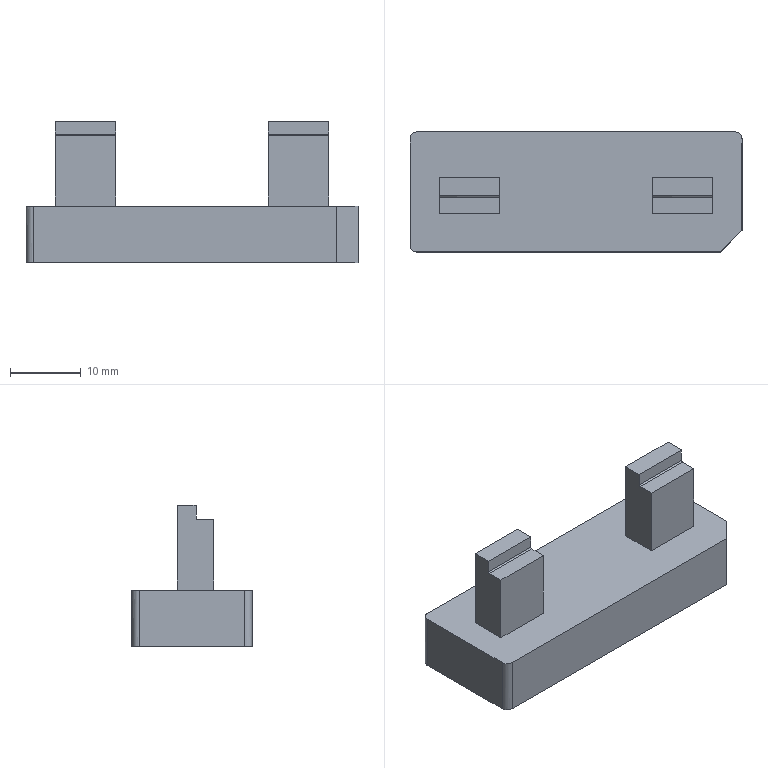NC program | PowerMill | posted by the shop | part box 47 x 17 x 19.985 mm
Lines 10964 to 11898 of 62704:
( TOOL ID   D10_1_1_1 )
( TOOL DIA. 10. TIP RAD 0 LENGTH 75.16 )
( Z = -2.265 )
T3 M6
T14
G91 G28 Z0
G0 G90 G54
M08
S8500 M3
X0 Y0 M8
G43 Z11.805 H3
X-.07 Y-.853
Z-1.065
G1 Z-2.265 F360
X-5.345 Y-.906 F600
G3 X-5.466 Y-1.223 I.478 J-.363
G1 X-5.474 Y-1.325
X-5.509 Y-1.6
X-5.56 Y-1.875
X-5.632 Y-2.177
X-5.706 Y-2.425
X-5.804 Y-2.7
X-5.918 Y-2.975
X-6.039 Y-3.227
X-6.177 Y-3.478
X-6.38 Y-3.8
X-6.581 Y-4.075
X-6.739 Y-4.268
X-6.814 Y-4.355
X-7.074 Y-4.625
X-7.3 Y-4.833
X-7.52 Y-5.013
X-7.739 Y-5.176
X-7.862 Y-5.259
X-8.143 Y-5.433
X-8.423 Y-5.583
X-8.734 Y-5.726
X-8.985 Y-5.824
X-9.266 Y-5.918
X-9.547 Y-5.995
X-9.827 Y-6.056
X-10.108 Y-6.101
X-10.389 Y-6.131
X-10.67 Y-6.146
X-19.374 Y-6.149
X-19.655 Y-6.139
X-19.935 Y-6.114
X-20.216 Y-6.074
X-20.497 Y-6.02
X-20.778 Y-5.949
X-21.059 Y-5.862
X-21.416 Y-5.726
X-21.658 Y-5.617
X-21.901 Y-5.492
X-22.156 Y-5.344
X-22.463 Y-5.139
X-22.743 Y-4.923
X-23.076 Y-4.625
X-23.339 Y-4.35
X-23.586 Y-4.054
X-23.777 Y-3.789
X-23.945 Y-3.525
X-24.099 Y-3.25
X-24.177 Y-3.093
X-24.249 Y-2.933
X-24.347 Y-2.697
X-24.444 Y-2.425
X-24.525 Y-2.15
X-24.563 Y-1.988
G3 X-24.805 Y-1.634 I-.584 J-.139
G0 Z4.005
G1 X-12.997 Y-11.339 F10000
G0 Z.935
G1 Z-.265 F360
X-12.996 Y-6.064 F600
X-12.957 Y-1.957
X-12.492 Y-1.961
G3 X-11.93 Y1.925 I.019 J1.981
G1 X-16.802 Y3.314
G3 X-19.35 Y1.366 I-.548 J-1.923
G1 X-19.334 Y.066
G3 X-17.356 Y-1.909 I2. J.025
G1 X-12.957 Y-1.957
X-12.996 Y-6.064
G0 Z5.789
G1 X30.08 Y-.856 F10000
G0 Z-1.065
G1 Z-2.265 F360
X24.805 Y-.908 F600
G3 X24.684 Y-1.225 I.477 J-.363
G1 X24.676 Y-1.325
X24.64 Y-1.6
X24.59 Y-1.875
X24.525 Y-2.15
X24.444 Y-2.425
X24.347 Y-2.698
X24.232 Y-2.975
X24.099 Y-3.25
X23.945 Y-3.525
X23.777 Y-3.79
X23.569 Y-4.075
X23.34 Y-4.35
X23.076 Y-4.625
X22.743 Y-4.923
X22.412 Y-5.176
X22.156 Y-5.344
X21.901 Y-5.492
X21.659 Y-5.617
X21.339 Y-5.758
X21.059 Y-5.862
X20.778 Y-5.949
X20.497 Y-6.02
X20.216 Y-6.075
X19.935 Y-6.115
X19.655 Y-6.139
X19.093 Y-6.149
X10.67 Y-6.147
X10.389 Y-6.131
X10.108 Y-6.101
X9.827 Y-6.056
X9.547 Y-5.995
X9.266 Y-5.918
X8.985 Y-5.825
X8.704 Y-5.713
X8.423 Y-5.583
X8.143 Y-5.433
X7.862 Y-5.259
X7.691 Y-5.142
X7.519 Y-5.014
X7.3 Y-4.834
X7.074 Y-4.625
X6.899 Y-4.447
X6.739 Y-4.269
X6.581 Y-4.075
X6.38 Y-3.8
X6.177 Y-3.479
X6.039 Y-3.227
X5.918 Y-2.975
X5.803 Y-2.7
X5.706 Y-2.425
X5.616 Y-2.113
X5.56 Y-1.875
X5.509 Y-1.6
X5.474 Y-1.325
X5.466 Y-1.229
G3 X5.345 Y-.911 I-.598 J-.047
G0 Z4.005
G1 X12.685 Y-11.339 F10000
G0 Z.935
G1 Z-.265 F360
X12.684 Y-6.064 F600
X12.552 Y-2.035
X17.415 Y-1.876
G3 X19.349 Y.139 I-.065 J1.999
G1 X19.339 Y1.422
G3 X17.378 Y3.405 I-2. J-.016
G1 X12.515 Y3.5
G3 X10.485 Y1.482 I-.039 J-1.991
G1 X10.506 Y-.082
G3 X12.552 Y-2.035 I1.981 J.026
G1 X12.684 Y-6.064
G0 Z11.805
X0 Y0
Z9.805
X34.255 Y2.994
Z-10.98
G1 Z-12.18 F360
X28.98 Y2.993 F600
X24.676 Y2.655
X24.698 Y2.374
X24.705 Y2.092
Y-3.092
X24.698 Y-3.374
X24.676 Y-3.655
X24.652 Y-3.838
X24.587 Y-4.211
G2 X24.442 Y-4.755 I-6.334 J1.406
G1 X24.348 Y-5.02
X24.24 Y-5.281
X24.119 Y-5.535
X23.984 Y-5.782
G2 X23.678 Y-6.255 I-5.425 J3.187
G1 X23.506 Y-6.478
X23.323 Y-6.692
X23.129 Y-6.897
X22.925 Y-7.09
X22.711 Y-7.273
X22.487 Y-7.445
G2 X22.015 Y-7.752 I-3.627 J5.068
G1 X21.73 Y-7.904
X21.513 Y-8.007
X21.253 Y-8.115
X20.988 Y-8.209
X20.717 Y-8.289
X20.444 Y-8.355
X20.167 Y-8.406
X19.887 Y-8.443
X19.607 Y-8.465
X19.325 Y-8.472
X10.825
X10.543 Y-8.465
G2 X9.983 Y-8.406 I.394 J6.44
X9.433 Y-8.289 I1.068 J6.378
G1 X9.237 Y-8.231
G2 X7.489 Y-7.312 I1.572 J5.11
G1 X7.439 Y-7.273
X7.225 Y-7.09
X7.021 Y-6.897
X6.827 Y-6.692
X6.644 Y-6.478
G2 X6.313 Y-6.023 I4.896 J3.905
G1 X6.216 Y-5.865
X6.031 Y-5.535
X5.91 Y-5.281
X5.802 Y-5.02
X5.708 Y-4.755
G2 X5.563 Y-4.211 I5.923 J1.878
X5.474 Y-3.655 I6.366 J1.293
G1 X5.452 Y-3.374
X5.445 Y-3.092
Y2.092
X5.452 Y2.374
X5.474 Y2.655
G2 X5.563 Y3.211 I6.451 J-.737
G1 X5.646 Y3.544
X1.04 Y4.907
G3 X.592 Y1.694 I10.461 J-3.096
G1 X.647 Y-3.314
G3 X1.62 Y-7.434 I10.155 J.221
G1 X1.929 Y-8.089
G2 X1.243 Y-9.172 I-.686 J-.325
G1 X-1.243
G2 X-1.923 Y-8.076 I0 J.759
G1 X-1.783 Y-7.792
G3 X-.557 Y-2.333 I-10.541 J5.233
G1 X-.647 Y2.316
G3 X-2.227 Y7.536 I-10.137 J-.219
G1 X-2.595 Y8.115
G2 X-2.013 Y9.174 I.582 J.37
G1 X2.005
G2 X2.581 Y8.1 I0 J-.691
G1 X2.412 Y7.846
G3 X1.04 Y4.907 I9.088 J-6.035
G1 X5.646 Y3.544
X5.708 Y3.755
X5.802 Y4.02
X5.91 Y4.281
G2 X6.166 Y4.782 I5.819 J-2.649
G1 X6.259 Y4.936
X6.357 Y5.087
X6.472 Y5.255
X6.644 Y5.478
X6.827 Y5.692
G2 X7.225 Y6.09 I4.744 J-4.346
X7.663 Y6.445 I4.211 J-4.753
G1 X7.954 Y6.64
X8.135 Y6.752
X8.383 Y6.886
X8.637 Y7.007
X8.897 Y7.115
X9.162 Y7.209
X9.433 Y7.289
X9.706 Y7.355
X9.983 Y7.406
X10.263 Y7.443
X10.543 Y7.465
X10.825 Y7.472
X19.325
G2 X19.887 Y7.443 I-.055 J-6.421
G1 X20.167 Y7.406
X20.444 Y7.355
X20.717 Y7.289
X20.988 Y7.209
X21.253 Y7.115
X21.513 Y7.007
X21.767 Y6.886
X22.015 Y6.752
X22.255 Y6.604
X22.487 Y6.445
X22.711 Y6.273
X22.925 Y6.09
G2 X23.323 Y5.692 I-4.355 J-4.753
G1 X23.506 Y5.478
X23.678 Y5.255
X23.837 Y5.023
X23.984 Y4.782
X24.119 Y4.535
X24.24 Y4.281
G2 X24.442 Y3.755 I-5.912 J-2.571
G1 X24.522 Y3.485
X24.565 Y3.307
X24.639 Y2.934
X24.676 Y2.655
X28.98 Y2.993
G0 Z2.9
G1 X-34.254 Y-3.753 F10000
G0 Z-10.98
G1 Z-12.18 F360
X-28.979 F600
X-24.693 Y-3.444
X-24.705 Y-3.092
Y2.093
X-24.698 Y2.374
X-24.676 Y2.655
X-24.639 Y2.934
X-24.587 Y3.211
G2 X-24.442 Y3.755 I6.134 J-1.352
X-24.24 Y4.281 I6.104 J-2.042
X-23.984 Y4.783 I5.883 J-2.681
G1 X-23.837 Y5.023
X-23.678 Y5.255
X-23.506 Y5.478
X-23.323 Y5.693
X-23.129 Y5.897
X-22.925 Y6.091
X-22.711 Y6.274
X-22.487 Y6.445
X-22.255 Y6.605
X-22.015 Y6.752
X-21.767 Y6.886
X-21.513 Y7.008
X-21.253 Y7.115
X-20.988 Y7.209
X-20.717 Y7.289
X-20.444 Y7.355
X-20.167 Y7.407
X-19.887 Y7.443
X-19.607 Y7.465
X-19.325 Y7.473
X-10.825
X-10.543 Y7.465
X-10.202 Y7.435
X-9.983 Y7.407
G2 X-9.433 Y7.289 I-1.05 J-6.292
X-8.897 Y7.115 I-1.734 J-6.247
G1 X-8.637 Y7.008
X-8.383 Y6.886
X-8.135 Y6.752
X-7.895 Y6.605
G2 X-7.439 Y6.274 I-3.483 J-5.273
G1 X-7.293 Y6.15
X-7.021 Y5.897
X-6.827 Y5.693
X-6.644 Y5.478
X-6.472 Y5.255
X-6.313 Y5.023
X-6.166 Y4.783
X-6.031 Y4.535
X-5.91 Y4.281
X-5.802 Y4.021
G2 X-5.628 Y3.485 I-6.041 J-2.259
G1 X-5.563 Y3.211
X-5.529 Y3.031
X-5.474 Y2.655
X-5.452 Y2.374
X-5.445 Y2.093
Y-3.092
X-5.452 Y-3.374
X-5.474 Y-3.654
X-5.511 Y-3.934
X-5.563 Y-4.211
X-5.628 Y-4.484
G2 X-5.802 Y-5.02 I-6.251 J1.735
G1 X-5.91 Y-5.28
X-6.031 Y-5.534
X-6.166 Y-5.782
X-6.313 Y-6.022
X-6.472 Y-6.254
X-6.644 Y-6.478
X-6.827 Y-6.692
G2 X-7.225 Y-7.09 I-4.584 J4.186
G1 X-7.439 Y-7.273
X-7.663 Y-7.445
X-7.895 Y-7.604
G2 X-8.383 Y-7.886 I-3.353 J5.244
G1 X-8.673 Y-8.022
X-8.897 Y-8.115
X-9.162 Y-8.209
X-9.433 Y-8.289
X-9.706 Y-8.354
X-9.983 Y-8.406
X-10.263 Y-8.443
X-10.543 Y-8.465
X-10.825 Y-8.472
X-19.325
X-19.607 Y-8.465
X-19.887 Y-8.443
G2 X-20.444 Y-8.354 I.736 J6.448
G1 X-20.717 Y-8.289
X-20.988 Y-8.209
X-21.253 Y-8.115
X-21.513 Y-8.007
X-21.767 Y-7.886
X-22.015 Y-7.751
X-22.255 Y-7.604
X-22.487 Y-7.444
X-22.711 Y-7.273
X-22.925 Y-7.09
G2 X-23.323 Y-6.692 I4.33 J4.728
X-23.678 Y-6.254 I4.857 J4.296
X-23.984 Y-5.782 I5.193 J3.708
G1 X-24.119 Y-5.534
X-24.24 Y-5.28
X-24.348 Y-5.02
X-24.442 Y-4.754
X-24.522 Y-4.484
G2 X-24.639 Y-3.934 I6.275 J1.622
G1 X-24.671 Y-3.689
X-24.693 Y-3.444
X-28.979 Y-3.753
G0 Z9.805
X0 Y0
X28.488 Y-14.767
Z-18.88
G1 Z-20.08 F360
G3 X24.953 Y-11.232 I-1.768 J1.768 F600
G1 X24.114 Y-12.07
Y-12.071
X24.113
X23.924 Y-12.252
X23.923 Y-12.254
X23.922 Y-12.255
X23.767 Y-12.39
X23.766 Y-12.391
X23.765 Y-12.392
X23.603 Y-12.522
X23.601 Y-12.524
X23.599 Y-12.525
X23.283 Y-12.75
X23.281 Y-12.751
X23.278 Y-12.753
X22.962 Y-12.944
X22.96 Y-12.945
X22.958 Y-12.946
X22.794 Y-13.033
X22.792
X22.791 Y-13.034
X22.639 Y-13.108
X22.637
X22.636 Y-13.109
X22.319 Y-13.243
X22.317 Y-13.244
X22.314 Y-13.245
X21.999 Y-13.354
X21.997 Y-13.355
X21.994
X21.677 Y-13.442
X21.674
X21.672 Y-13.443
X21.356 Y-13.507
X21.353 Y-13.508
X21.351
X21.035 Y-13.552
X21.032
X21.03
X20.713 Y-13.575
X20.711 Y-13.576
X20.709
X20.392 Y-13.58
X20.391
X-22.288
X-22.289
X-22.605 Y-13.579
X-22.606
X-22.608
X-22.924 Y-13.565
X-22.926
X-22.928
X-23.244 Y-13.534
X-23.247
X-23.249
X-23.565 Y-13.486
X-23.567
X-23.569 Y-13.485
X-23.885 Y-13.42
X-23.887
X-23.889 Y-13.419
X-24.136 Y-13.356
X-24.138 Y-13.355
X-24.14 Y-13.354
X-24.525 Y-13.232
X-24.528
X-24.53 Y-13.231
X-24.846 Y-13.109
X-24.848 Y-13.108
X-24.849
X-25.015 Y-13.035
X-25.016
X-25.017 Y-13.034
X-25.168 Y-12.963
X-25.169 Y-12.962
X-25.171
X-25.487 Y-12.796
X-25.488 Y-12.795
X-25.49 Y-12.794
X-25.626 Y-12.715
X-25.627 Y-12.714
X-25.628
X-25.808 Y-12.601
X-25.81 Y-12.6
X-25.811 Y-12.599
X-26.106 Y-12.395
X-26.108 Y-12.394
X-26.11 Y-12.392
X-26.448 Y-12.124
X-26.45 Y-12.122
X-26.452 Y-12.12
X-26.768 Y-11.83
X-26.77 Y-11.828
X-26.771 Y-11.827
X-26.844 Y-11.754
X-26.845 Y-11.753
X-26.846 Y-11.752
X-27.089 Y-11.488
X-27.091 Y-11.486
X-27.093 Y-11.484
X-27.388 Y-11.115
X-27.39 Y-11.113
X-27.392 Y-11.111
X-27.61 Y-10.794
X-27.611 Y-10.793
X-27.612 Y-10.791
X-27.731 Y-10.599
Y-10.598
X-27.732 Y-10.597
X-27.804 Y-10.473
Y-10.471
X-27.805 Y-10.47
X-27.97 Y-10.154
X-27.971 Y-10.152
X-27.972 Y-10.149
X-28.114 Y-9.833
X-28.115 Y-9.831
X-28.116 Y-9.829
X-28.237 Y-9.513
X-28.238 Y-9.511
X-28.239 Y-9.509
X-28.34 Y-9.193
Y-9.19
X-28.341 Y-9.188
X-28.423 Y-8.872
X-28.424 Y-8.87
Y-8.868
X-28.488 Y-8.552
Y-8.55
Y-8.548
X-28.536 Y-8.232
Y-8.229
Y-8.227
X-28.565 Y-7.911
Y-7.909
X-28.566 Y-7.907
X-28.579 Y-7.591
Y-7.589
Y-7.587
Y7.587
Y7.589
Y7.591
X-28.566 Y7.907
Y7.909
Y7.911
X-28.536 Y8.227
Y8.229
Y8.231
X-28.489 Y8.548
Y8.55
X-28.488 Y8.552
X-28.424 Y8.868
Y8.87
X-28.423 Y8.872
X-28.341 Y9.188
X-28.34 Y9.19
Y9.193
X-28.238 Y9.509
Y9.511
X-28.237 Y9.513
X-28.116 Y9.829
Y9.831
X-28.115 Y9.832
X-28.052 Y9.977
Y9.979
X-28.051 Y9.98
X-27.972 Y10.15
X-27.971 Y10.152
X-27.97 Y10.154
X-27.805 Y10.47
X-27.804 Y10.471
Y10.473
X-27.732 Y10.597
X-27.731 Y10.598
Y10.599
X-27.612 Y10.791
X-27.611 Y10.793
X-27.61 Y10.794
X-27.413 Y11.082
X-27.411 Y11.084
X-27.409 Y11.086
X-27.138 Y11.431
X-27.137 Y11.433
X-27.135 Y11.435
X-26.846 Y11.751
X-26.845 Y11.753
X-26.844 Y11.754
X-26.771 Y11.827
X-26.77 Y11.828
X-26.769 Y11.829
X-26.508 Y12.072
X-26.505 Y12.074
X-26.503 Y12.076
X-26.132 Y12.376
X-26.13 Y12.377
X-26.128 Y12.379
X-25.811 Y12.599
X-25.81 Y12.6
X-25.808 Y12.601
X-25.628 Y12.714
X-25.627
X-25.626 Y12.715
X-25.49 Y12.794
X-25.488 Y12.795
X-25.487 Y12.796
X-25.171 Y12.962
X-25.169 Y12.963
X-25.168
X-25.017 Y13.034
X-25.016 Y13.035
X-25.015
X-24.849 Y13.108
X-24.848
X-24.846 Y13.109
X-24.53 Y13.231
X-24.528 Y13.232
X-24.526
X-24.21 Y13.335
X-24.208
X-24.206 Y13.336
X-23.889 Y13.419
X-23.887 Y13.42
X-23.885
X-23.569 Y13.485
X-23.567
X-23.565
X-23.249 Y13.534
X-23.247
X-23.244
X-22.928 Y13.564
X-22.926
X-22.924 Y13.565
X-22.608 Y13.579
X-22.606
X-22.605
X-22.289 Y13.58
X-22.288
X0
X22.288
X22.289
X22.605 Y13.579
X22.606
X22.608
X22.924 Y13.565
X22.926
X22.928
X23.244 Y13.534
X23.247
X23.249
X23.565 Y13.486
X23.567
X23.569 Y13.485
X23.885 Y13.42
X23.887
X23.889 Y13.419
X24.136 Y13.356
X24.138 Y13.355
X24.14 Y13.354
X24.525 Y13.232
X24.528
X24.53 Y13.231
X24.846 Y13.109
X24.848 Y13.108
X24.849
X25.015 Y13.035
X25.016
X25.017 Y13.034
X25.168 Y12.963
X25.169 Y12.962
X25.171
X25.487 Y12.796
X25.488 Y12.795
X25.49 Y12.794
X25.626 Y12.715
X25.627 Y12.714
X25.628
X25.808 Y12.601
X25.81 Y12.6
X25.811 Y12.599
X26.106 Y12.395
X26.108 Y12.394
X26.11 Y12.392
X26.448 Y12.124
X26.45 Y12.122
X26.452 Y12.12
X26.768 Y11.83
X26.77 Y11.828
X26.771 Y11.827
X26.844 Y11.754
X26.845 Y11.753
X26.846 Y11.752
X27.089 Y11.488
X27.091 Y11.486
X27.093 Y11.484
X27.388 Y11.115
X27.39 Y11.113
X27.392 Y11.111
X27.61 Y10.794
X27.611 Y10.793
X27.612 Y10.791
X27.731 Y10.599
Y10.598
X27.732 Y10.597
X27.804 Y10.473
Y10.471
X27.805 Y10.47
X27.97 Y10.154
X27.971 Y10.152
X27.972 Y10.149
X28.114 Y9.833
X28.115 Y9.831
X28.116 Y9.829
X28.237 Y9.513
X28.238 Y9.511
X28.239 Y9.509
X28.34 Y9.193
Y9.19
X28.341 Y9.188
X28.423 Y8.872
X28.424 Y8.87
Y8.868
X28.488 Y8.552
Y8.55
Y8.548
X28.536 Y8.232
Y8.229
Y8.227
X28.565 Y7.911
Y7.909
X28.566 Y7.907
X28.579 Y7.591
Y7.589
Y7.588
X28.58 Y-5.374
Y-5.375
X28.576 Y-5.692
Y-5.694
Y-5.696
X28.554 Y-6.012
Y-6.015
Y-6.017
X28.511 Y-6.334
Y-6.336
X28.51 Y-6.339
X28.447 Y-6.655
X28.446 Y-6.657
Y-6.66
X28.372 Y-6.937
Y-6.94
X28.371 Y-6.942
X28.252 Y-7.297
X28.251 Y-7.3
X28.25 Y-7.302
X28.117 Y-7.618
X28.116 Y-7.62
Y-7.622
X28.051 Y-7.757
X28.05 Y-7.758
Y-7.76
X27.955 Y-7.941
X27.954 Y-7.943
X27.953 Y-7.945
X27.764 Y-8.261
X27.763 Y-8.263
X27.761 Y-8.266
X27.538 Y-8.582
X27.537 Y-8.584
X27.535 Y-8.586
X27.409 Y-8.744
X27.408 Y-8.745
X27.407 Y-8.747
X27.27 Y-8.904
X27.269 Y-8.906
X27.268 Y-8.907
X27.088 Y-9.096
X27.087 Y-9.097
X24.953 Y-11.232
G3 X28.488 Y-14.767 I1.768 J-1.768
G1 X28.437 Y-14.705
G3 X24.901 Y-11.17 I-1.768 J1.768
G1 X24.058 Y-12.014
X23.869 Y-12.195
X23.715 Y-12.33
X23.553 Y-12.46
X23.237 Y-12.685
X22.921 Y-12.875
X22.756 Y-12.962
X22.604 Y-13.036
X22.288 Y-13.169
X21.973 Y-13.278
X21.656 Y-13.365
X21.34 Y-13.429
X21.024 Y-13.473
X20.708 Y-13.496
X20.391 Y-13.5
X-22.288
X-22.604 Y-13.499
X-22.921 Y-13.485
X-23.237 Y-13.455
X-23.553 Y-13.407
X-23.869 Y-13.342
X-24.116 Y-13.278
X-24.501 Y-13.156
X-24.817 Y-13.034
X-24.983 Y-12.962
X-25.134 Y-12.891
X-25.45 Y-12.725
X-25.585 Y-12.646
X-25.766 Y-12.533
X-26.06 Y-12.33
X-26.398 Y-12.061
X-26.714 Y-11.771
X-26.787 Y-11.697
X-27.03 Y-11.434
X-27.326 Y-11.065
X-27.544 Y-10.749
X-27.663 Y-10.557
X-27.734 Y-10.433
X-27.899 Y-10.117
X-28.041 Y-9.801
X-28.162 Y-9.484
X-28.263 Y-9.168
X-28.346 Y-8.852
X-28.409 Y-8.536
X-28.457 Y-8.22
X-28.486 Y-7.904
X-28.499 Y-7.587
X-28.5 Y-7.271
Y7.271
X-28.499 Y7.587
X-28.486 Y7.904
X-28.457 Y8.22
X-28.41 Y8.536
X-28.346 Y8.852
X-28.263 Y9.168
X-28.162 Y9.484
X-28.041 Y9.801
X-27.979 Y9.946
X-27.899 Y10.117
X-27.734 Y10.433
X-27.663 Y10.557
X-27.544 Y10.749
X-27.347 Y11.037
X-27.076 Y11.381
X-26.787 Y11.697
X-26.714 Y11.771
X-26.453 Y12.014
X-26.082 Y12.313
X-25.766 Y12.533
X-25.585 Y12.646
X-25.45 Y12.725
X-25.134 Y12.891
X-24.983 Y12.962
X-24.817 Y13.034
X-24.501 Y13.156
X-24.185 Y13.258
X-23.869 Y13.342
X-23.553 Y13.406
X-23.237 Y13.455
X-22.921 Y13.485
X-22.604 Y13.499
X-22.288 Y13.5
X0
X22.288
X22.604 Y13.499
X22.921 Y13.485
X23.237 Y13.455
X23.553 Y13.407
X23.869 Y13.342
X24.116 Y13.278
X24.501 Y13.156
X24.817 Y13.034
X24.983 Y12.962
X25.134 Y12.891
X25.45 Y12.725
X25.585 Y12.646
X25.766 Y12.533
X26.06 Y12.33
X26.398 Y12.061
X26.714 Y11.771
X26.787 Y11.697
X27.03 Y11.434
X27.326 Y11.065
X27.544 Y10.749
X27.663 Y10.557
X27.734 Y10.433
X27.899 Y10.117
X28.041 Y9.801
X28.162 Y9.484
X28.263 Y9.168
X28.346 Y8.852
X28.409 Y8.536
X28.457 Y8.22
X28.486 Y7.904
X28.499 Y7.587
X28.5 Y7.271
Y-5.374
X28.496 Y-5.691
X28.474 Y-6.007
X28.432 Y-6.323
X28.369 Y-6.639
X28.295 Y-6.917
X28.176 Y-7.271
X28.043 Y-7.587
X27.979 Y-7.723
X27.884 Y-7.904
X27.696 Y-8.22
X27.473 Y-8.536
X27.347 Y-8.694
X27.21 Y-8.852
X27.03 Y-9.041
X24.901 Y-11.17
G3 X28.437 Y-14.705 I1.768 J-1.768
G0 Z9.805
Z10.805
X0 Y0
M9
M5
M01